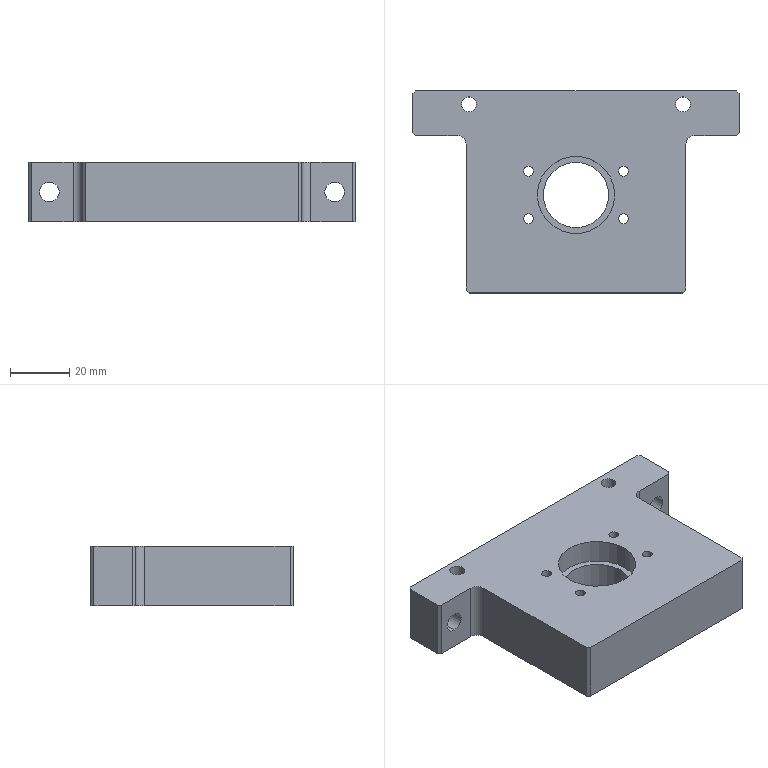Part | STEP file | Bearing mounting plate 2 | 1 solid | 39 faces | box 110 x 68 x 20 mm | volume 100152 mm3 | cylinder 22 | plane 17 | commonest cylinder face diameters 3.3 x8 5 x4 6.6 x4 6 x2 22 x2 26 x2